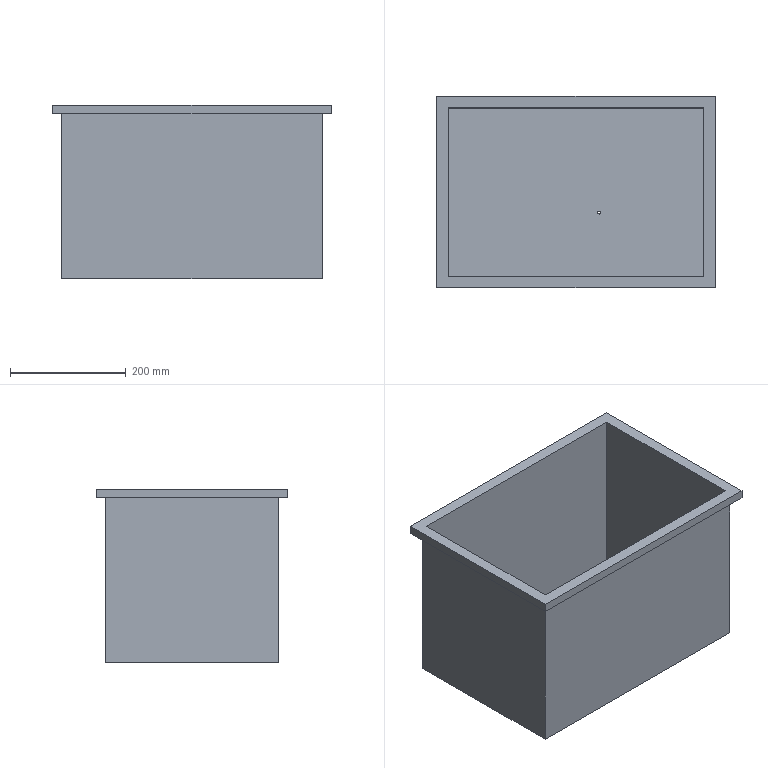Part | STEP file | Material box | 1 solid | 18 faces | box 480 x 330 x 300 mm | volume 3208902 mm3 | plane 16 | cylinder 2 | commonest cylinder face diameters 5 x2
STEP:
#1=CARTESIAN_POINT('',(0.,0.,0.));
#2=DIRECTION('',(0.,0.,1.));
#3=DIRECTION('',(1.,0.,0.));
#4=AXIS2_PLACEMENT_3D('',#1,#2,#3);
#5=CARTESIAN_POINT('',(42.5,-35.,0.));
#6=VERTEX_POINT('',#5);
#7=CARTESIAN_POINT('',(42.5,-35.,5.));
#8=VERTEX_POINT('',#7);
#9=CARTESIAN_POINT('',(42.5,-35.,-5.));
#10=DIRECTION('',(0.,0.,1.));
#11=VECTOR('',#10,1.);
#12=LINE('',#9,#11);
#13=CARTESIAN_POINT('',(40.,-35.,-5.));
#14=DIRECTION('',(0.,0.,1.));
#15=DIRECTION('',(1.,0.,0.));
#16=AXIS2_PLACEMENT_3D('',#13,#14,#15);
#17=CYLINDRICAL_SURFACE('',#16,2.5);
#18=CARTESIAN_POINT('',(6.283,0.));
#19=DIRECTION('',(0.,1.));
#20=VECTOR('',#19,1.);
#21=LINE('',#18,#20);
#22=(GEOMETRIC_REPRESENTATION_CONTEXT(2)PARAMETRIC_REPRESENTATION_CONTEXT()REPRESENTATION_CONTEXT('',''));
#23=DEFINITIONAL_REPRESENTATION('',(#21),#22);
#24=PCURVE('',#17,#23);
#25=CARTESIAN_POINT('',(40.,-35.,-5.));
#26=DIRECTION('',(0.,0.,1.));
#27=DIRECTION('',(1.,0.,0.));
#28=AXIS2_PLACEMENT_3D('',#25,#26,#27);
#29=CYLINDRICAL_SURFACE('',#28,2.5);
#30=CARTESIAN_POINT('',(0.,0.));
#31=DIRECTION('',(0.,1.));
#32=VECTOR('',#31,1.);
#33=LINE('',#30,#32);
#34=(GEOMETRIC_REPRESENTATION_CONTEXT(2)PARAMETRIC_REPRESENTATION_CONTEXT()REPRESENTATION_CONTEXT('',''));
#35=DEFINITIONAL_REPRESENTATION('',(#33),#34);
#36=PCURVE('',#29,#35);
#37=SURFACE_CURVE('',#12,(#24,#36),.PCURVE_S1.);
#38=EDGE_CURVE('',#6,#8,#37,.T.);
#39=ORIENTED_EDGE('',*,*,#38,.T.);
#40=CARTESIAN_POINT('',(37.5,-35.,5.));
#41=VERTEX_POINT('',#40);
#42=CARTESIAN_POINT('',(40.,-35.,5.));
#43=DIRECTION('',(0.,0.,-1.));
#44=DIRECTION('',(1.,0.,0.));
#45=AXIS2_PLACEMENT_3D('',#42,#43,#44);
#46=CIRCLE('',#45,2.5);
#47=CARTESIAN_POINT('',(6.283,10.));
#48=DIRECTION('',(-1.,0.));
#49=VECTOR('',#48,1.);
#50=LINE('',#47,#49);
#51=(GEOMETRIC_REPRESENTATION_CONTEXT(2)PARAMETRIC_REPRESENTATION_CONTEXT()REPRESENTATION_CONTEXT('',''));
#52=DEFINITIONAL_REPRESENTATION('',(#50),#51);
#53=PCURVE('',#17,#52);
#54=CARTESIAN_POINT('',(0.,0.,5.));
#55=DIRECTION('',(0.,0.,1.));
#56=DIRECTION('',(1.,0.,0.));
#57=AXIS2_PLACEMENT_3D('',#54,#55,#56);
#58=PLANE('',#57);
#59=CARTESIAN_POINT('',(42.5,-35.));
#60=CARTESIAN_POINT('',(42.5,-39.33));
#61=CARTESIAN_POINT('',(38.75,-37.165));
#62=CARTESIAN_POINT('',(35.,-35.));
#63=CARTESIAN_POINT('',(38.75,-32.835));
#64=CARTESIAN_POINT('',(42.5,-30.67));
#65=CARTESIAN_POINT('',(42.5,-35.));
#66=(BOUNDED_CURVE()B_SPLINE_CURVE(2,(#59,#60,#61,#62,#63,#64,#65),.UNSPECIFIED.,.T.,.F.)B_SPLINE_CURVE_WITH_KNOTS((1,2,2,2,2,1),(-2.094,0.,2.094,4.189,6.283,8.378),.UNSPECIFIED.)CURVE()GEOMETRIC_REPRESENTATION_ITEM()RATIONAL_B_SPLINE_CURVE((1.,0.5,1.,0.5,1.,0.5,1.))REPRESENTATION_ITEM(''));
#67=(GEOMETRIC_REPRESENTATION_CONTEXT(2)PARAMETRIC_REPRESENTATION_CONTEXT()REPRESENTATION_CONTEXT('',''));
#68=DEFINITIONAL_REPRESENTATION('',(#66),#67);
#69=PCURVE('',#58,#68);
#70=SURFACE_CURVE('',#46,(#53,#69),.PCURVE_S1.);
#71=EDGE_CURVE('',#8,#41,#70,.T.);
#72=ORIENTED_EDGE('',*,*,#71,.T.);
#73=CARTESIAN_POINT('',(37.5,-35.,0.));
#74=VERTEX_POINT('',#73);
#75=CARTESIAN_POINT('',(37.5,-35.,-5.));
#76=DIRECTION('',(0.,0.,1.));
#77=VECTOR('',#76,1.);
#78=LINE('',#75,#77);
#79=CARTESIAN_POINT('',(3.142,0.));
#80=DIRECTION('',(0.,1.));
#81=VECTOR('',#80,1.);
#82=LINE('',#79,#81);
#83=(GEOMETRIC_REPRESENTATION_CONTEXT(2)PARAMETRIC_REPRESENTATION_CONTEXT()REPRESENTATION_CONTEXT('',''));
#84=DEFINITIONAL_REPRESENTATION('',(#82),#83);
#85=PCURVE('',#17,#84);
#86=CARTESIAN_POINT('',(3.142,0.));
#87=DIRECTION('',(0.,1.));
#88=VECTOR('',#87,1.);
#89=LINE('',#86,#88);
#90=(GEOMETRIC_REPRESENTATION_CONTEXT(2)PARAMETRIC_REPRESENTATION_CONTEXT()REPRESENTATION_CONTEXT('',''));
#91=DEFINITIONAL_REPRESENTATION('',(#89),#90);
#92=PCURVE('',#29,#91);
#93=SURFACE_CURVE('',#78,(#85,#92),.PCURVE_S1.);
#94=EDGE_CURVE('',#74,#41,#93,.T.);
#95=ORIENTED_EDGE('',*,*,#94,.F.);
#96=CARTESIAN_POINT('',(40.,-35.,0.));
#97=DIRECTION('',(0.,0.,-1.));
#98=DIRECTION('',(1.,0.,0.));
#99=AXIS2_PLACEMENT_3D('',#96,#97,#98);
#100=CIRCLE('',#99,2.5);
#101=CARTESIAN_POINT('',(6.283,5.));
#102=DIRECTION('',(-1.,0.));
#103=VECTOR('',#102,1.);
#104=LINE('',#101,#103);
#105=(GEOMETRIC_REPRESENTATION_CONTEXT(2)PARAMETRIC_REPRESENTATION_CONTEXT()REPRESENTATION_CONTEXT('',''));
#106=DEFINITIONAL_REPRESENTATION('',(#104),#105);
#107=PCURVE('',#17,#106);
#108=CARTESIAN_POINT('',(0.,0.,0.));
#109=DIRECTION('',(0.,0.,1.));
#110=DIRECTION('',(1.,0.,0.));
#111=AXIS2_PLACEMENT_3D('',#108,#109,#110);
#112=PLANE('',#111);
#113=CARTESIAN_POINT('',(42.5,-35.));
#114=CARTESIAN_POINT('',(42.5,-39.33));
#115=CARTESIAN_POINT('',(38.75,-37.165));
#116=CARTESIAN_POINT('',(35.,-35.));
#117=CARTESIAN_POINT('',(38.75,-32.835));
#118=CARTESIAN_POINT('',(42.5,-30.67));
#119=CARTESIAN_POINT('',(42.5,-35.));
#120=(BOUNDED_CURVE()B_SPLINE_CURVE(2,(#113,#114,#115,#116,#117,#118,#119),.UNSPECIFIED.,.T.,.F.)B_SPLINE_CURVE_WITH_KNOTS((1,2,2,2,2,1),(-2.094,0.,2.094,4.189,6.283,8.378),.UNSPECIFIED.)CURVE()GEOMETRIC_REPRESENTATION_ITEM()RATIONAL_B_SPLINE_CURVE((1.,0.5,1.,0.5,1.,0.5,1.))REPRESENTATION_ITEM(''));
#121=(GEOMETRIC_REPRESENTATION_CONTEXT(2)PARAMETRIC_REPRESENTATION_CONTEXT()REPRESENTATION_CONTEXT('',''));
#122=DEFINITIONAL_REPRESENTATION('',(#120),#121);
#123=PCURVE('',#112,#122);
#124=SURFACE_CURVE('',#100,(#107,#123),.PCURVE_S1.);
#125=EDGE_CURVE('',#6,#74,#124,.T.);
#126=ORIENTED_EDGE('',*,*,#125,.F.);
#127=EDGE_LOOP('',(#39,#72,#95,#126));
#128=FACE_BOUND('',#127,.F.);
#129=ADVANCED_FACE('',(#128),#17,.F.);
#130=CARTESIAN_POINT('',(-225.,-150.,0.));
#131=VERTEX_POINT('',#130);
#132=CARTESIAN_POINT('',(225.,-150.,0.));
#133=VERTEX_POINT('',#132);
#134=CARTESIAN_POINT('',(0.,-150.,0.));
#135=DIRECTION('',(1.,0.,0.));
#136=VECTOR('',#135,1.);
#137=LINE('',#134,#136);
#138=CARTESIAN_POINT('',(0.,-150.));
#139=DIRECTION('',(1.,0.));
#140=VECTOR('',#139,1.);
#141=LINE('',#138,#140);
#142=(GEOMETRIC_REPRESENTATION_CONTEXT(2)PARAMETRIC_REPRESENTATION_CONTEXT()REPRESENTATION_CONTEXT('',''));
#143=DEFINITIONAL_REPRESENTATION('',(#141),#142);
#144=PCURVE('',#112,#143);
#145=CARTESIAN_POINT('',(-225.,-150.,300.));
#146=DIRECTION('',(0.,1.,0.));
#147=DIRECTION('',(0.,0.,1.));
#148=AXIS2_PLACEMENT_3D('',#145,#146,#147);
#149=PLANE('',#148);
#150=CARTESIAN_POINT('',(-300.,225.));
#151=DIRECTION('',(0.,1.));
#152=VECTOR('',#151,1.);
#153=LINE('',#150,#152);
#154=(GEOMETRIC_REPRESENTATION_CONTEXT(2)PARAMETRIC_REPRESENTATION_CONTEXT()REPRESENTATION_CONTEXT('',''));
#155=DEFINITIONAL_REPRESENTATION('',(#153),#154);
#156=PCURVE('',#149,#155);
#157=SURFACE_CURVE('',#137,(#144,#156),.PCURVE_S1.);
#158=EDGE_CURVE('',#131,#133,#157,.T.);
#159=ORIENTED_EDGE('',*,*,#158,.F.);
#160=CARTESIAN_POINT('',(-225.,150.,0.));
#161=VERTEX_POINT('',#160);
#162=CARTESIAN_POINT('',(-225.,0.,0.));
#163=DIRECTION('',(0.,-1.,0.));
#164=VECTOR('',#163,1.);
#165=LINE('',#162,#164);
#166=CARTESIAN_POINT('',(-225.,0.));
#167=DIRECTION('',(0.,-1.));
#168=VECTOR('',#167,1.);
#169=LINE('',#166,#168);
#170=(GEOMETRIC_REPRESENTATION_CONTEXT(2)PARAMETRIC_REPRESENTATION_CONTEXT()REPRESENTATION_CONTEXT('',''));
#171=DEFINITIONAL_REPRESENTATION('',(#169),#170);
#172=PCURVE('',#112,#171);
#173=CARTESIAN_POINT('',(-225.,150.,300.));
#174=DIRECTION('',(1.,0.,0.));
#175=DIRECTION('',(0.,1.,0.));
#176=AXIS2_PLACEMENT_3D('',#173,#174,#175);
#177=PLANE('',#176);
#178=CARTESIAN_POINT('',(-150.,-300.));
#179=DIRECTION('',(-1.,0.));
#180=VECTOR('',#179,1.);
#181=LINE('',#178,#180);
#182=(GEOMETRIC_REPRESENTATION_CONTEXT(2)PARAMETRIC_REPRESENTATION_CONTEXT()REPRESENTATION_CONTEXT('',''));
#183=DEFINITIONAL_REPRESENTATION('',(#181),#182);
#184=PCURVE('',#177,#183);
#185=SURFACE_CURVE('',#165,(#172,#184),.PCURVE_S1.);
#186=EDGE_CURVE('',#161,#131,#185,.T.);
#187=ORIENTED_EDGE('',*,*,#186,.F.);
#188=CARTESIAN_POINT('',(225.,150.,0.));
#189=VERTEX_POINT('',#188);
#190=CARTESIAN_POINT('',(0.,150.,0.));
#191=DIRECTION('',(-1.,0.,0.));
#192=VECTOR('',#191,1.);
#193=LINE('',#190,#192);
#194=CARTESIAN_POINT('',(0.,150.));
#195=DIRECTION('',(-1.,0.));
#196=VECTOR('',#195,1.);
#197=LINE('',#194,#196);
#198=(GEOMETRIC_REPRESENTATION_CONTEXT(2)PARAMETRIC_REPRESENTATION_CONTEXT()REPRESENTATION_CONTEXT('',''));
#199=DEFINITIONAL_REPRESENTATION('',(#197),#198);
#200=PCURVE('',#112,#199);
#201=CARTESIAN_POINT('',(-225.,150.,300.));
#202=DIRECTION('',(0.,-1.,0.));
#203=DIRECTION('',(0.,0.,-1.));
#204=AXIS2_PLACEMENT_3D('',#201,#202,#203);
#205=PLANE('',#204);
#206=CARTESIAN_POINT('',(300.,225.));
#207=DIRECTION('',(0.,-1.));
#208=VECTOR('',#207,1.);
#209=LINE('',#206,#208);
#210=(GEOMETRIC_REPRESENTATION_CONTEXT(2)PARAMETRIC_REPRESENTATION_CONTEXT()REPRESENTATION_CONTEXT('',''));
#211=DEFINITIONAL_REPRESENTATION('',(#209),#210);
#212=PCURVE('',#205,#211);
#213=SURFACE_CURVE('',#193,(#200,#212),.PCURVE_S1.);
#214=EDGE_CURVE('',#189,#161,#213,.T.);
#215=ORIENTED_EDGE('',*,*,#214,.F.);
#216=CARTESIAN_POINT('',(225.,0.,0.));
#217=DIRECTION('',(0.,1.,0.));
#218=VECTOR('',#217,1.);
#219=LINE('',#216,#218);
#220=CARTESIAN_POINT('',(225.,0.));
#221=DIRECTION('',(0.,1.));
#222=VECTOR('',#221,1.);
#223=LINE('',#220,#222);
#224=(GEOMETRIC_REPRESENTATION_CONTEXT(2)PARAMETRIC_REPRESENTATION_CONTEXT()REPRESENTATION_CONTEXT('',''));
#225=DEFINITIONAL_REPRESENTATION('',(#223),#224);
#226=PCURVE('',#112,#225);
#227=CARTESIAN_POINT('',(225.,150.,300.));
#228=DIRECTION('',(-1.,0.,0.));
#229=DIRECTION('',(0.,-1.,0.));
#230=AXIS2_PLACEMENT_3D('',#227,#228,#229);
#231=PLANE('',#230);
#232=CARTESIAN_POINT('',(150.,-300.));
#233=DIRECTION('',(-1.,0.));
#234=VECTOR('',#233,1.);
#235=LINE('',#232,#234);
#236=(GEOMETRIC_REPRESENTATION_CONTEXT(2)PARAMETRIC_REPRESENTATION_CONTEXT()REPRESENTATION_CONTEXT('',''));
#237=DEFINITIONAL_REPRESENTATION('',(#235),#236);
#238=PCURVE('',#231,#237);
#239=SURFACE_CURVE('',#219,(#226,#238),.PCURVE_S1.);
#240=EDGE_CURVE('',#133,#189,#239,.T.);
#241=ORIENTED_EDGE('',*,*,#240,.F.);
#242=EDGE_LOOP('',(#159,#187,#215,#241));
#243=FACE_BOUND('',#242,.T.);
#244=ORIENTED_EDGE('',*,*,#125,.F.);
#245=CARTESIAN_POINT('',(40.,-35.,0.));
#246=DIRECTION('',(0.,0.,-1.));
#247=DIRECTION('',(1.,0.,0.));
#248=AXIS2_PLACEMENT_3D('',#245,#246,#247);
#249=CIRCLE('',#248,2.5);
#250=CARTESIAN_POINT('',(42.5,-35.));
#251=CARTESIAN_POINT('',(42.5,-39.33));
#252=CARTESIAN_POINT('',(38.75,-37.165));
#253=CARTESIAN_POINT('',(35.,-35.));
#254=CARTESIAN_POINT('',(38.75,-32.835));
#255=CARTESIAN_POINT('',(42.5,-30.67));
#256=CARTESIAN_POINT('',(42.5,-35.));
#257=(BOUNDED_CURVE()B_SPLINE_CURVE(2,(#250,#251,#252,#253,#254,#255,#256),.UNSPECIFIED.,.T.,.F.)B_SPLINE_CURVE_WITH_KNOTS((1,2,2,2,2,1),(-2.094,0.,2.094,4.189,6.283,8.378),.UNSPECIFIED.)CURVE()GEOMETRIC_REPRESENTATION_ITEM()RATIONAL_B_SPLINE_CURVE((1.,0.5,1.,0.5,1.,0.5,1.))REPRESENTATION_ITEM(''));
#258=(GEOMETRIC_REPRESENTATION_CONTEXT(2)PARAMETRIC_REPRESENTATION_CONTEXT()REPRESENTATION_CONTEXT('',''));
#259=DEFINITIONAL_REPRESENTATION('',(#257),#258);
#260=PCURVE('',#112,#259);
#261=CARTESIAN_POINT('',(6.283,5.));
#262=DIRECTION('',(-1.,0.));
#263=VECTOR('',#262,1.);
#264=LINE('',#261,#263);
#265=(GEOMETRIC_REPRESENTATION_CONTEXT(2)PARAMETRIC_REPRESENTATION_CONTEXT()REPRESENTATION_CONTEXT('',''));
#266=DEFINITIONAL_REPRESENTATION('',(#264),#265);
#267=PCURVE('',#29,#266);
#268=SURFACE_CURVE('',#249,(#260,#267),.PCURVE_S1.);
#269=EDGE_CURVE('',#74,#6,#268,.T.);
#270=ORIENTED_EDGE('',*,*,#269,.F.);
#271=EDGE_LOOP('',(#244,#270));
#272=FACE_BOUND('',#271,.T.);
#273=ADVANCED_FACE('',(#243,#272),#112,.F.);
#274=CARTESIAN_POINT('',(225.,-150.,285.));
#275=VERTEX_POINT('',#274);
#276=CARTESIAN_POINT('',(225.,150.,285.));
#277=VERTEX_POINT('',#276);
#278=CARTESIAN_POINT('',(225.,150.,285.));
#279=DIRECTION('',(0.,1.,0.));
#280=VECTOR('',#279,1.);
#281=LINE('',#278,#280);
#282=CARTESIAN_POINT('',(0.,-15.));
#283=DIRECTION('',(-1.,0.));
#284=VECTOR('',#283,1.);
#285=LINE('',#282,#284);
#286=(GEOMETRIC_REPRESENTATION_CONTEXT(2)PARAMETRIC_REPRESENTATION_CONTEXT()REPRESENTATION_CONTEXT('',''));
#287=DEFINITIONAL_REPRESENTATION('',(#285),#286);
#288=PCURVE('',#231,#287);
#289=CARTESIAN_POINT('',(0.,0.,285.));
#290=DIRECTION('',(0.,0.,-1.));
#291=DIRECTION('',(-1.,0.,0.));
#292=AXIS2_PLACEMENT_3D('',#289,#290,#291);
#293=PLANE('',#292);
#294=CARTESIAN_POINT('',(-225.,150.));
#295=DIRECTION('',(0.,1.));
#296=VECTOR('',#295,1.);
#297=LINE('',#294,#296);
#298=(GEOMETRIC_REPRESENTATION_CONTEXT(2)PARAMETRIC_REPRESENTATION_CONTEXT()REPRESENTATION_CONTEXT('',''));
#299=DEFINITIONAL_REPRESENTATION('',(#297),#298);
#300=PCURVE('',#293,#299);
#301=SURFACE_CURVE('',#281,(#288,#300),.PCURVE_S1.);
#302=EDGE_CURVE('',#275,#277,#301,.T.);
#303=ORIENTED_EDGE('',*,*,#302,.F.);
#304=CARTESIAN_POINT('',(225.,-150.,300.));
#305=DIRECTION('',(0.,0.,1.));
#306=VECTOR('',#305,1.);
#307=LINE('',#304,#306);
#308=CARTESIAN_POINT('',(300.,0.));
#309=DIRECTION('',(0.,1.));
#310=VECTOR('',#309,1.);
#311=LINE('',#308,#310);
#312=(GEOMETRIC_REPRESENTATION_CONTEXT(2)PARAMETRIC_REPRESENTATION_CONTEXT()REPRESENTATION_CONTEXT('',''));
#313=DEFINITIONAL_REPRESENTATION('',(#311),#312);
#314=PCURVE('',#231,#313);
#315=CARTESIAN_POINT('',(0.,450.));
#316=DIRECTION('',(1.,0.));
#317=VECTOR('',#316,1.);
#318=LINE('',#315,#317);
#319=(GEOMETRIC_REPRESENTATION_CONTEXT(2)PARAMETRIC_REPRESENTATION_CONTEXT()REPRESENTATION_CONTEXT('',''));
#320=DEFINITIONAL_REPRESENTATION('',(#318),#319);
#321=PCURVE('',#149,#320);
#322=SURFACE_CURVE('',#307,(#314,#321),.PCURVE_S1.);
#323=EDGE_CURVE('',#133,#275,#322,.T.);
#324=ORIENTED_EDGE('',*,*,#323,.F.);
#325=ORIENTED_EDGE('',*,*,#240,.T.);
#326=CARTESIAN_POINT('',(225.,150.,300.));
#327=DIRECTION('',(0.,0.,-1.));
#328=VECTOR('',#327,1.);
#329=LINE('',#326,#328);
#330=CARTESIAN_POINT('',(0.,0.));
#331=DIRECTION('',(0.,-1.));
#332=VECTOR('',#331,1.);
#333=LINE('',#330,#332);
#334=(GEOMETRIC_REPRESENTATION_CONTEXT(2)PARAMETRIC_REPRESENTATION_CONTEXT()REPRESENTATION_CONTEXT('',''));
#335=DEFINITIONAL_REPRESENTATION('',(#333),#334);
#336=PCURVE('',#231,#335);
#337=CARTESIAN_POINT('',(0.,450.));
#338=DIRECTION('',(1.,0.));
#339=VECTOR('',#338,1.);
#340=LINE('',#337,#339);
#341=(GEOMETRIC_REPRESENTATION_CONTEXT(2)PARAMETRIC_REPRESENTATION_CONTEXT()REPRESENTATION_CONTEXT('',''));
#342=DEFINITIONAL_REPRESENTATION('',(#340),#341);
#343=PCURVE('',#205,#342);
#344=SURFACE_CURVE('',#329,(#336,#343),.PCURVE_S1.);
#345=EDGE_CURVE('',#277,#189,#344,.T.);
#346=ORIENTED_EDGE('',*,*,#345,.F.);
#347=EDGE_LOOP('',(#303,#324,#325,#346));
#348=FACE_BOUND('',#347,.T.);
#349=ADVANCED_FACE('',(#348),#231,.F.);
#350=CARTESIAN_POINT('',(-225.,-150.,285.));
#351=VERTEX_POINT('',#350);
#352=CARTESIAN_POINT('',(-225.,-150.,285.));
#353=DIRECTION('',(1.,0.,0.));
#354=VECTOR('',#353,1.);
#355=LINE('',#352,#354);
#356=CARTESIAN_POINT('',(-15.,0.));
#357=DIRECTION('',(0.,1.));
#358=VECTOR('',#357,1.);
#359=LINE('',#356,#358);
#360=(GEOMETRIC_REPRESENTATION_CONTEXT(2)PARAMETRIC_REPRESENTATION_CONTEXT()REPRESENTATION_CONTEXT('',''));
#361=DEFINITIONAL_REPRESENTATION('',(#359),#360);
#362=PCURVE('',#149,#361);
#363=CARTESIAN_POINT('',(225.,-150.));
#364=DIRECTION('',(-1.,0.));
#365=VECTOR('',#364,1.);
#366=LINE('',#363,#365);
#367=(GEOMETRIC_REPRESENTATION_CONTEXT(2)PARAMETRIC_REPRESENTATION_CONTEXT()REPRESENTATION_CONTEXT('',''));
#368=DEFINITIONAL_REPRESENTATION('',(#366),#367);
#369=PCURVE('',#293,#368);
#370=SURFACE_CURVE('',#355,(#362,#369),.PCURVE_S1.);
#371=EDGE_CURVE('',#351,#275,#370,.T.);
#372=ORIENTED_EDGE('',*,*,#371,.F.);
#373=CARTESIAN_POINT('',(-225.,-150.,300.));
#374=DIRECTION('',(0.,0.,1.));
#375=VECTOR('',#374,1.);
#376=LINE('',#373,#375);
#377=CARTESIAN_POINT('',(0.,0.));
#378=DIRECTION('',(1.,0.));
#379=VECTOR('',#378,1.);
#380=LINE('',#377,#379);
#381=(GEOMETRIC_REPRESENTATION_CONTEXT(2)PARAMETRIC_REPRESENTATION_CONTEXT()REPRESENTATION_CONTEXT('',''));
#382=DEFINITIONAL_REPRESENTATION('',(#380),#381);
#383=PCURVE('',#149,#382);
#384=CARTESIAN_POINT('',(-300.,0.));
#385=DIRECTION('',(0.,1.));
#386=VECTOR('',#385,1.);
#387=LINE('',#384,#386);
#388=(GEOMETRIC_REPRESENTATION_CONTEXT(2)PARAMETRIC_REPRESENTATION_CONTEXT()REPRESENTATION_CONTEXT('',''));
#389=DEFINITIONAL_REPRESENTATION('',(#387),#388);
#390=PCURVE('',#177,#389);
#391=SURFACE_CURVE('',#376,(#383,#390),.PCURVE_S1.);
#392=EDGE_CURVE('',#131,#351,#391,.T.);
#393=ORIENTED_EDGE('',*,*,#392,.F.);
#394=ORIENTED_EDGE('',*,*,#158,.T.);
#395=ORIENTED_EDGE('',*,*,#323,.T.);
#396=EDGE_LOOP('',(#372,#393,#394,#395));
#397=FACE_BOUND('',#396,.T.);
#398=ADVANCED_FACE('',(#397),#149,.F.);
#399=CARTESIAN_POINT('',(-225.,150.,285.));
#400=VERTEX_POINT('',#399);
#401=CARTESIAN_POINT('',(-225.,150.,285.));
#402=DIRECTION('',(0.,-1.,0.));
#403=VECTOR('',#402,1.);
#404=LINE('',#401,#403);
#405=CARTESIAN_POINT('',(0.,-15.));
#406=DIRECTION('',(-1.,0.));
#407=VECTOR('',#406,1.);
#408=LINE('',#405,#407);
#409=(GEOMETRIC_REPRESENTATION_CONTEXT(2)PARAMETRIC_REPRESENTATION_CONTEXT()REPRESENTATION_CONTEXT('',''));
#410=DEFINITIONAL_REPRESENTATION('',(#408),#409);
#411=PCURVE('',#177,#410);
#412=CARTESIAN_POINT('',(225.,150.));
#413=DIRECTION('',(0.,-1.));
#414=VECTOR('',#413,1.);
#415=LINE('',#412,#414);
#416=(GEOMETRIC_REPRESENTATION_CONTEXT(2)PARAMETRIC_REPRESENTATION_CONTEXT()REPRESENTATION_CONTEXT('',''));
#417=DEFINITIONAL_REPRESENTATION('',(#415),#416);
#418=PCURVE('',#293,#417);
#419=SURFACE_CURVE('',#404,(#411,#418),.PCURVE_S1.);
#420=EDGE_CURVE('',#400,#351,#419,.T.);
#421=ORIENTED_EDGE('',*,*,#420,.F.);
#422=CARTESIAN_POINT('',(-225.,150.,300.));
#423=DIRECTION('',(0.,0.,1.));
#424=VECTOR('',#423,1.);
#425=LINE('',#422,#424);
#426=CARTESIAN_POINT('',(0.,0.));
#427=DIRECTION('',(0.,1.));
#428=VECTOR('',#427,1.);
#429=LINE('',#426,#428);
#430=(GEOMETRIC_REPRESENTATION_CONTEXT(2)PARAMETRIC_REPRESENTATION_CONTEXT()REPRESENTATION_CONTEXT('',''));
#431=DEFINITIONAL_REPRESENTATION('',(#429),#430);
#432=PCURVE('',#177,#431);
#433=CARTESIAN_POINT('',(0.,0.));
#434=DIRECTION('',(-1.,0.));
#435=VECTOR('',#434,1.);
#436=LINE('',#433,#435);
#437=(GEOMETRIC_REPRESENTATION_CONTEXT(2)PARAMETRIC_REPRESENTATION_CONTEXT()REPRESENTATION_CONTEXT('',''));
#438=DEFINITIONAL_REPRESENTATION('',(#436),#437);
#439=PCURVE('',#205,#438);
#440=SURFACE_CURVE('',#425,(#432,#439),.PCURVE_S1.);
#441=EDGE_CURVE('',#161,#400,#440,.T.);
#442=ORIENTED_EDGE('',*,*,#441,.F.);
#443=ORIENTED_EDGE('',*,*,#186,.T.);
#444=ORIENTED_EDGE('',*,*,#392,.T.);
#445=EDGE_LOOP('',(#421,#442,#443,#444));
#446=FACE_BOUND('',#445,.T.);
#447=ADVANCED_FACE('',(#446),#177,.F.);
#448=CARTESIAN_POINT('',(-225.,150.,285.));
#449=DIRECTION('',(-1.,0.,0.));
#450=VECTOR('',#449,1.);
#451=LINE('',#448,#450);
#452=CARTESIAN_POINT('',(15.,0.));
#453=DIRECTION('',(0.,-1.));
#454=VECTOR('',#453,1.);
#455=LINE('',#452,#454);
#456=(GEOMETRIC_REPRESENTATION_CONTEXT(2)PARAMETRIC_REPRESENTATION_CONTEXT()REPRESENTATION_CONTEXT('',''));
#457=DEFINITIONAL_REPRESENTATION('',(#455),#456);
#458=PCURVE('',#205,#457);
#459=CARTESIAN_POINT('',(225.,150.));
#460=DIRECTION('',(1.,0.));
#461=VECTOR('',#460,1.);
#462=LINE('',#459,#461);
#463=(GEOMETRIC_REPRESENTATION_CONTEXT(2)PARAMETRIC_REPRESENTATION_CONTEXT()REPRESENTATION_CONTEXT('',''));
#464=DEFINITIONAL_REPRESENTATION('',(#462),#463);
#465=PCURVE('',#293,#464);
#466=SURFACE_CURVE('',#451,(#458,#465),.PCURVE_S1.);
#467=EDGE_CURVE('',#277,#400,#466,.T.);
#468=ORIENTED_EDGE('',*,*,#467,.F.);
#469=ORIENTED_EDGE('',*,*,#345,.T.);
#470=ORIENTED_EDGE('',*,*,#214,.T.);
#471=ORIENTED_EDGE('',*,*,#441,.T.);
#472=EDGE_LOOP('',(#468,#469,#470,#471));
#473=FACE_BOUND('',#472,.T.);
#474=ADVANCED_FACE('',(#473),#205,.F.);
#475=CARTESIAN_POINT('',(40.,-35.,5.));
#476=DIRECTION('',(0.,0.,-1.));
#477=DIRECTION('',(1.,0.,0.));
#478=AXIS2_PLACEMENT_3D('',#475,#476,#477);
#479=CIRCLE('',#478,2.5);
#480=CARTESIAN_POINT('',(6.283,10.));
#481=DIRECTION('',(-1.,0.));
#482=VECTOR('',#481,1.);
#483=LINE('',#480,#482);
#484=(GEOMETRIC_REPRESENTATION_CONTEXT(2)PARAMETRIC_REPRESENTATION_CONTEXT()REPRESENTATION_CONTEXT('',''));
#485=DEFINITIONAL_REPRESENTATION('',(#483),#484);
#486=PCURVE('',#29,#485);
#487=CARTESIAN_POINT('',(42.5,-35.));
#488=CARTESIAN_POINT('',(42.5,-39.33));
#489=CARTESIAN_POINT('',(38.75,-37.165));
#490=CARTESIAN_POINT('',(35.,-35.));
#491=CARTESIAN_POINT('',(38.75,-32.835));
#492=CARTESIAN_POINT('',(42.5,-30.67));
#493=CARTESIAN_POINT('',(42.5,-35.));
#494=(BOUNDED_CURVE()B_SPLINE_CURVE(2,(#487,#488,#489,#490,#491,#492,#493),.UNSPECIFIED.,.T.,.F.)B_SPLINE_CURVE_WITH_KNOTS((1,2,2,2,2,1),(-2.094,0.,2.094,4.189,6.283,8.378),.UNSPECIFIED.)CURVE()GEOMETRIC_REPRESENTATION_ITEM()RATIONAL_B_SPLINE_CURVE((1.,0.5,1.,0.5,1.,0.5,1.))REPRESENTATION_ITEM(''));
#495=(GEOMETRIC_REPRESENTATION_CONTEXT(2)PARAMETRIC_REPRESENTATION_CONTEXT()REPRESENTATION_CONTEXT('',''));
#496=DEFINITIONAL_REPRESENTATION('',(#494),#495);
#497=PCURVE('',#58,#496);
#498=SURFACE_CURVE('',#479,(#486,#497),.PCURVE_S1.);
#499=EDGE_CURVE('',#41,#8,#498,.T.);
#500=ORIENTED_EDGE('',*,*,#499,.T.);
#501=ORIENTED_EDGE('',*,*,#38,.F.);
#502=ORIENTED_EDGE('',*,*,#269,.F.);
#503=ORIENTED_EDGE('',*,*,#94,.T.);
#504=EDGE_LOOP('',(#500,#501,#502,#503));
#505=FACE_BOUND('',#504,.F.);
#506=ADVANCED_FACE('',(#505),#29,.F.);
#507=CARTESIAN_POINT('',(240.,-165.,285.));
#508=VERTEX_POINT('',#507);
#509=CARTESIAN_POINT('',(-240.,-165.,285.));
#510=VERTEX_POINT('',#509);
#511=CARTESIAN_POINT('',(0.,-165.,285.));
#512=DIRECTION('',(-1.,0.,0.));
#513=VECTOR('',#512,1.);
#514=LINE('',#511,#513);
#515=CARTESIAN_POINT('',(0.,-165.));
#516=DIRECTION('',(1.,0.));
#517=VECTOR('',#516,1.);
#518=LINE('',#515,#517);
#519=(GEOMETRIC_REPRESENTATION_CONTEXT(2)PARAMETRIC_REPRESENTATION_CONTEXT()REPRESENTATION_CONTEXT('',''));
#520=DEFINITIONAL_REPRESENTATION('',(#518),#519);
#521=PCURVE('',#293,#520);
#522=CARTESIAN_POINT('',(-240.,-165.,285.));
#523=DIRECTION('',(0.,-1.,0.));
#524=DIRECTION('',(0.,0.,-1.));
#525=AXIS2_PLACEMENT_3D('',#522,#523,#524);
#526=PLANE('',#525);
#527=CARTESIAN_POINT('',(0.,240.));
#528=DIRECTION('',(0.,-1.));
#529=VECTOR('',#528,1.);
#530=LINE('',#527,#529);
#531=(GEOMETRIC_REPRESENTATION_CONTEXT(2)PARAMETRIC_REPRESENTATION_CONTEXT()REPRESENTATION_CONTEXT('',''));
#532=DEFINITIONAL_REPRESENTATION('',(#530),#531);
#533=PCURVE('',#526,#532);
#534=SURFACE_CURVE('',#514,(#521,#533),.PCURVE_S1.);
#535=EDGE_CURVE('',#508,#510,#534,.T.);
#536=ORIENTED_EDGE('',*,*,#535,.T.);
#537=CARTESIAN_POINT('',(-240.,165.,285.));
#538=VERTEX_POINT('',#537);
#539=CARTESIAN_POINT('',(-240.,0.,285.));
#540=DIRECTION('',(0.,1.,0.));
#541=VECTOR('',#540,1.);
#542=LINE('',#539,#541);
#543=CARTESIAN_POINT('',(240.,0.));
#544=DIRECTION('',(0.,1.));
#545=VECTOR('',#544,1.);
#546=LINE('',#543,#545);
#547=(GEOMETRIC_REPRESENTATION_CONTEXT(2)PARAMETRIC_REPRESENTATION_CONTEXT()REPRESENTATION_CONTEXT('',''));
#548=DEFINITIONAL_REPRESENTATION('',(#546),#547);
#549=PCURVE('',#293,#548);
#550=CARTESIAN_POINT('',(-240.,165.,285.));
#551=DIRECTION('',(-1.,0.,0.));
#552=DIRECTION('',(0.,-1.,0.));
#553=AXIS2_PLACEMENT_3D('',#550,#551,#552);
#554=PLANE('',#553);
#555=CARTESIAN_POINT('',(165.,0.));
#556=DIRECTION('',(-1.,0.));
#557=VECTOR('',#556,1.);
#558=LINE('',#555,#557);
#559=(GEOMETRIC_REPRESENTATION_CONTEXT(2)PARAMETRIC_REPRESENTATION_CONTEXT()REPRESENTATION_CONTEXT('',''));
#560=DEFINITIONAL_REPRESENTATION('',(#558),#559);
#561=PCURVE('',#554,#560);
#562=SURFACE_CURVE('',#542,(#549,#561),.PCURVE_S1.);
#563=EDGE_CURVE('',#510,#538,#562,.T.);
#564=ORIENTED_EDGE('',*,*,#563,.T.);
#565=CARTESIAN_POINT('',(240.,165.,285.));
#566=VERTEX_POINT('',#565);
#567=CARTESIAN_POINT('',(0.,165.,285.));
#568=DIRECTION('',(1.,0.,0.));
#569=VECTOR('',#568,1.);
#570=LINE('',#567,#569);
#571=CARTESIAN_POINT('',(0.,165.));
#572=DIRECTION('',(-1.,0.));
#573=VECTOR('',#572,1.);
#574=LINE('',#571,#573);
#575=(GEOMETRIC_REPRESENTATION_CONTEXT(2)PARAMETRIC_REPRESENTATION_CONTEXT()REPRESENTATION_CONTEXT('',''));
#576=DEFINITIONAL_REPRESENTATION('',(#574),#575);
#577=PCURVE('',#293,#576);
#578=CARTESIAN_POINT('',(-240.,165.,285.));
#579=DIRECTION('',(0.,1.,0.));
#580=DIRECTION('',(0.,0.,1.));
#581=AXIS2_PLACEMENT_3D('',#578,#579,#580);
#582=PLANE('',#581);
#583=CARTESIAN_POINT('',(0.,240.));
#584=DIRECTION('',(0.,1.));
#585=VECTOR('',#584,1.);
#586=LINE('',#583,#585);
#587=(GEOMETRIC_REPRESENTATION_CONTEXT(2)PARAMETRIC_REPRESENTATION_CONTEXT()REPRESENTATION_CONTEXT('',''));
#588=DEFINITIONAL_REPRESENTATION('',(#586),#587);
#589=PCURVE('',#582,#588);
#590=SURFACE_CURVE('',#570,(#577,#589),.PCURVE_S1.);
#591=EDGE_CURVE('',#538,#566,#590,.T.);
#592=ORIENTED_EDGE('',*,*,#591,.T.);
#593=CARTESIAN_POINT('',(240.,0.,285.));
#594=DIRECTION('',(0.,-1.,0.));
#595=VECTOR('',#594,1.);
#596=LINE('',#593,#595);
#597=CARTESIAN_POINT('',(-240.,0.));
#598=DIRECTION('',(0.,-1.));
#599=VECTOR('',#598,1.);
#600=LINE('',#597,#599);
#601=(GEOMETRIC_REPRESENTATION_CONTEXT(2)PARAMETRIC_REPRESENTATION_CONTEXT()REPRESENTATION_CONTEXT('',''));
#602=DEFINITIONAL_REPRESENTATION('',(#600),#601);
#603=PCURVE('',#293,#602);
#604=CARTESIAN_POINT('',(240.,165.,285.));
#605=DIRECTION('',(1.,0.,0.));
#606=DIRECTION('',(0.,0.,-1.));
#607=AXIS2_PLACEMENT_3D('',#604,#605,#606);
#608=PLANE('',#607);
#609=CARTESIAN_POINT('',(0.,-165.));
#610=DIRECTION('',(0.,-1.));
#611=VECTOR('',#610,1.);
#612=LINE('',#609,#611);
#613=(GEOMETRIC_REPRESENTATION_CONTEXT(2)PARAMETRIC_REPRESENTATION_CONTEXT()REPRESENTATION_CONTEXT('',''));
#614=DEFINITIONAL_REPRESENTATION('',(#612),#613);
#615=PCURVE('',#608,#614);
#616=SURFACE_CURVE('',#596,(#603,#615),.PCURVE_S1.);
#617=EDGE_CURVE('',#566,#508,#616,.T.);
#618=ORIENTED_EDGE('',*,*,#617,.T.);
#619=EDGE_LOOP('',(#536,#564,#592,#618));
#620=FACE_BOUND('',#619,.T.);
#621=ORIENTED_EDGE('',*,*,#302,.T.);
#622=ORIENTED_EDGE('',*,*,#467,.T.);
#623=ORIENTED_EDGE('',*,*,#420,.T.);
#624=ORIENTED_EDGE('',*,*,#371,.T.);
#625=EDGE_LOOP('',(#621,#622,#623,#624));
#626=FACE_BOUND('',#625,.T.);
#627=ADVANCED_FACE('',(#620,#626),#293,.T.);
#628=CARTESIAN_POINT('',(-220.,145.,5.));
#629=VERTEX_POINT('',#628);
#630=CARTESIAN_POINT('',(-220.,-145.,5.));
#631=VERTEX_POINT('',#630);
#632=CARTESIAN_POINT('',(-220.,0.,5.));
#633=DIRECTION('',(0.,-1.,0.));
#634=VECTOR('',#633,1.);
#635=LINE('',#632,#634);
#636=CARTESIAN_POINT('',(-220.,0.));
#637=DIRECTION('',(0.,-1.));
#638=VECTOR('',#637,1.);
#639=LINE('',#636,#638);
#640=(GEOMETRIC_REPRESENTATION_CONTEXT(2)PARAMETRIC_REPRESENTATION_CONTEXT()REPRESENTATION_CONTEXT('',''));
#641=DEFINITIONAL_REPRESENTATION('',(#639),#640);
#642=PCURVE('',#58,#641);
#643=CARTESIAN_POINT('',(-220.,150.,300.));
#644=DIRECTION('',(1.,0.,0.));
#645=DIRECTION('',(0.,1.,0.));
#646=AXIS2_PLACEMENT_3D('',#643,#644,#645);
#647=PLANE('',#646);
#648=CARTESIAN_POINT('',(-150.,-295.));
#649=DIRECTION('',(-1.,0.));
#650=VECTOR('',#649,1.);
#651=LINE('',#648,#650);
#652=(GEOMETRIC_REPRESENTATION_CONTEXT(2)PARAMETRIC_REPRESENTATION_CONTEXT()REPRESENTATION_CONTEXT('',''));
#653=DEFINITIONAL_REPRESENTATION('',(#651),#652);
#654=PCURVE('',#647,#653);
#655=SURFACE_CURVE('',#635,(#642,#654),.PCURVE_S1.);
#656=EDGE_CURVE('',#629,#631,#655,.T.);
#657=ORIENTED_EDGE('',*,*,#656,.T.);
#658=CARTESIAN_POINT('',(220.,-145.,5.));
#659=VERTEX_POINT('',#658);
#660=CARTESIAN_POINT('',(0.,-145.,5.));
#661=DIRECTION('',(1.,0.,0.));
#662=VECTOR('',#661,1.);
#663=LINE('',#660,#662);
#664=CARTESIAN_POINT('',(0.,-145.));
#665=DIRECTION('',(1.,0.));
#666=VECTOR('',#665,1.);
#667=LINE('',#664,#666);
#668=(GEOMETRIC_REPRESENTATION_CONTEXT(2)PARAMETRIC_REPRESENTATION_CONTEXT()REPRESENTATION_CONTEXT('',''));
#669=DEFINITIONAL_REPRESENTATION('',(#667),#668);
#670=PCURVE('',#58,#669);
#671=CARTESIAN_POINT('',(-225.,-145.,300.));
#672=DIRECTION('',(0.,1.,0.));
#673=DIRECTION('',(0.,0.,1.));
#674=AXIS2_PLACEMENT_3D('',#671,#672,#673);
#675=PLANE('',#674);
#676=CARTESIAN_POINT('',(-295.,225.));
#677=DIRECTION('',(0.,1.));
#678=VECTOR('',#677,1.);
#679=LINE('',#676,#678);
#680=(GEOMETRIC_REPRESENTATION_CONTEXT(2)PARAMETRIC_REPRESENTATION_CONTEXT()REPRESENTATION_CONTEXT('',''));
#681=DEFINITIONAL_REPRESENTATION('',(#679),#680);
#682=PCURVE('',#675,#681);
#683=SURFACE_CURVE('',#663,(#670,#682),.PCURVE_S1.);
#684=EDGE_CURVE('',#631,#659,#683,.T.);
#685=ORIENTED_EDGE('',*,*,#684,.T.);
#686=CARTESIAN_POINT('',(220.,145.,5.));
#687=VERTEX_POINT('',#686);
#688=CARTESIAN_POINT('',(220.,0.,5.));
#689=DIRECTION('',(0.,1.,0.));
#690=VECTOR('',#689,1.);
#691=LINE('',#688,#690);
#692=CARTESIAN_POINT('',(220.,0.));
#693=DIRECTION('',(0.,1.));
#694=VECTOR('',#693,1.);
#695=LINE('',#692,#694);
#696=(GEOMETRIC_REPRESENTATION_CONTEXT(2)PARAMETRIC_REPRESENTATION_CONTEXT()REPRESENTATION_CONTEXT('',''));
#697=DEFINITIONAL_REPRESENTATION('',(#695),#696);
#698=PCURVE('',#58,#697);
#699=CARTESIAN_POINT('',(220.,150.,300.));
#700=DIRECTION('',(-1.,0.,0.));
#701=DIRECTION('',(0.,-1.,0.));
#702=AXIS2_PLACEMENT_3D('',#699,#700,#701);
#703=PLANE('',#702);
#704=CARTESIAN_POINT('',(150.,-295.));
#705=DIRECTION('',(-1.,0.));
#706=VECTOR('',#705,1.);
#707=LINE('',#704,#706);
#708=(GEOMETRIC_REPRESENTATION_CONTEXT(2)PARAMETRIC_REPRESENTATION_CONTEXT()REPRESENTATION_CONTEXT('',''));
#709=DEFINITIONAL_REPRESENTATION('',(#707),#708);
#710=PCURVE('',#703,#709);
#711=SURFACE_CURVE('',#691,(#698,#710),.PCURVE_S1.);
#712=EDGE_CURVE('',#659,#687,#711,.T.);
#713=ORIENTED_EDGE('',*,*,#712,.T.);
#714=CARTESIAN_POINT('',(0.,145.,5.));
#715=DIRECTION('',(-1.,0.,0.));
#716=VECTOR('',#715,1.);
#717=LINE('',#714,#716);
#718=CARTESIAN_POINT('',(0.,145.));
#719=DIRECTION('',(-1.,0.));
#720=VECTOR('',#719,1.);
#721=LINE('',#718,#720);
#722=(GEOMETRIC_REPRESENTATION_CONTEXT(2)PARAMETRIC_REPRESENTATION_CONTEXT()REPRESENTATION_CONTEXT('',''));
#723=DEFINITIONAL_REPRESENTATION('',(#721),#722);
#724=PCURVE('',#58,#723);
#725=CARTESIAN_POINT('',(-225.,145.,300.));
#726=DIRECTION('',(0.,-1.,0.));
#727=DIRECTION('',(0.,0.,-1.));
#728=AXIS2_PLACEMENT_3D('',#725,#726,#727);
#729=PLANE('',#728);
#730=CARTESIAN_POINT('',(295.,225.));
#731=DIRECTION('',(0.,-1.));
#732=VECTOR('',#731,1.);
#733=LINE('',#730,#732);
#734=(GEOMETRIC_REPRESENTATION_CONTEXT(2)PARAMETRIC_REPRESENTATION_CONTEXT()REPRESENTATION_CONTEXT('',''));
#735=DEFINITIONAL_REPRESENTATION('',(#733),#734);
#736=PCURVE('',#729,#735);
#737=SURFACE_CURVE('',#717,(#724,#736),.PCURVE_S1.);
#738=EDGE_CURVE('',#687,#629,#737,.T.);
#739=ORIENTED_EDGE('',*,*,#738,.T.);
#740=EDGE_LOOP('',(#657,#685,#713,#739));
#741=FACE_BOUND('',#740,.T.);
#742=ORIENTED_EDGE('',*,*,#71,.T.);
#743=ORIENTED_EDGE('',*,*,#499,.T.);
#744=EDGE_LOOP('',(#742,#743));
#745=FACE_BOUND('',#744,.T.);
#746=ADVANCED_FACE('',(#741,#745),#58,.T.);
#747=ORIENTED_EDGE('',*,*,#563,.F.);
#748=CARTESIAN_POINT('',(-240.,-165.,300.));
#749=VERTEX_POINT('',#748);
#750=CARTESIAN_POINT('',(-240.,-165.,285.));
#751=DIRECTION('',(0.,0.,1.));
#752=VECTOR('',#751,1.);
#753=LINE('',#750,#752);
#754=CARTESIAN_POINT('',(330.,0.));
#755=DIRECTION('',(0.,1.));
#756=VECTOR('',#755,1.);
#757=LINE('',#754,#756);
#758=(GEOMETRIC_REPRESENTATION_CONTEXT(2)PARAMETRIC_REPRESENTATION_CONTEXT()REPRESENTATION_CONTEXT('',''));
#759=DEFINITIONAL_REPRESENTATION('',(#757),#758);
#760=PCURVE('',#554,#759);
#761=CARTESIAN_POINT('',(0.,0.));
#762=DIRECTION('',(-1.,0.));
#763=VECTOR('',#762,1.);
#764=LINE('',#761,#763);
#765=(GEOMETRIC_REPRESENTATION_CONTEXT(2)PARAMETRIC_REPRESENTATION_CONTEXT()REPRESENTATION_CONTEXT('',''));
#766=DEFINITIONAL_REPRESENTATION('',(#764),#765);
#767=PCURVE('',#526,#766);
#768=SURFACE_CURVE('',#753,(#760,#767),.PCURVE_S1.);
#769=EDGE_CURVE('',#510,#749,#768,.T.);
#770=ORIENTED_EDGE('',*,*,#769,.T.);
#771=CARTESIAN_POINT('',(-240.,165.,300.));
#772=VERTEX_POINT('',#771);
#773=CARTESIAN_POINT('',(-240.,165.,300.));
#774=DIRECTION('',(0.,1.,0.));
#775=VECTOR('',#774,1.);
#776=LINE('',#773,#775);
#777=CARTESIAN_POINT('',(0.,15.));
#778=DIRECTION('',(-1.,0.));
#779=VECTOR('',#778,1.);
#780=LINE('',#777,#779);
#781=(GEOMETRIC_REPRESENTATION_CONTEXT(2)PARAMETRIC_REPRESENTATION_CONTEXT()REPRESENTATION_CONTEXT('',''));
#782=DEFINITIONAL_REPRESENTATION('',(#780),#781);
#783=PCURVE('',#554,#782);
#784=CARTESIAN_POINT('',(0.,0.,300.));
#785=DIRECTION('',(0.,0.,1.));
#786=DIRECTION('',(1.,0.,0.));
#787=AXIS2_PLACEMENT_3D('',#784,#785,#786);
#788=PLANE('',#787);
#789=CARTESIAN_POINT('',(-240.,165.));
#790=DIRECTION('',(0.,1.));
#791=VECTOR('',#790,1.);
#792=LINE('',#789,#791);
#793=(GEOMETRIC_REPRESENTATION_CONTEXT(2)PARAMETRIC_REPRESENTATION_CONTEXT()REPRESENTATION_CONTEXT('',''));
#794=DEFINITIONAL_REPRESENTATION('',(#792),#793);
#795=PCURVE('',#788,#794);
#796=SURFACE_CURVE('',#776,(#783,#795),.PCURVE_S1.);
#797=EDGE_CURVE('',#749,#772,#796,.T.);
#798=ORIENTED_EDGE('',*,*,#797,.T.);
#799=CARTESIAN_POINT('',(-240.,165.,285.));
#800=DIRECTION('',(0.,0.,-1.));
#801=VECTOR('',#800,1.);
#802=LINE('',#799,#801);
#803=CARTESIAN_POINT('',(0.,0.));
#804=DIRECTION('',(0.,-1.));
#805=VECTOR('',#804,1.);
#806=LINE('',#803,#805);
#807=(GEOMETRIC_REPRESENTATION_CONTEXT(2)PARAMETRIC_REPRESENTATION_CONTEXT()REPRESENTATION_CONTEXT('',''));
#808=DEFINITIONAL_REPRESENTATION('',(#806),#807);
#809=PCURVE('',#554,#808);
#810=CARTESIAN_POINT('',(0.,0.));
#811=DIRECTION('',(-1.,0.));
#812=VECTOR('',#811,1.);
#813=LINE('',#810,#812);
#814=(GEOMETRIC_REPRESENTATION_CONTEXT(2)PARAMETRIC_REPRESENTATION_CONTEXT()REPRESENTATION_CONTEXT('',''));
#815=DEFINITIONAL_REPRESENTATION('',(#813),#814);
#816=PCURVE('',#582,#815);
#817=SURFACE_CURVE('',#802,(#809,#816),.PCURVE_S1.);
#818=EDGE_CURVE('',#772,#538,#817,.T.);
#819=ORIENTED_EDGE('',*,*,#818,.T.);
#820=EDGE_LOOP('',(#747,#770,#798,#819));
#821=FACE_BOUND('',#820,.T.);
#822=ADVANCED_FACE('',(#821),#554,.T.);
#823=ORIENTED_EDGE('',*,*,#535,.F.);
#824=CARTESIAN_POINT('',(240.,-165.,300.));
#825=VERTEX_POINT('',#824);
#826=CARTESIAN_POINT('',(240.,-165.,285.));
#827=DIRECTION('',(0.,0.,1.));
#828=VECTOR('',#827,1.);
#829=LINE('',#826,#828);
#830=CARTESIAN_POINT('',(0.,480.));
#831=DIRECTION('',(-1.,0.));
#832=VECTOR('',#831,1.);
#833=LINE('',#830,#832);
#834=(GEOMETRIC_REPRESENTATION_CONTEXT(2)PARAMETRIC_REPRESENTATION_CONTEXT()REPRESENTATION_CONTEXT('',''));
#835=DEFINITIONAL_REPRESENTATION('',(#833),#834);
#836=PCURVE('',#526,#835);
#837=CARTESIAN_POINT('',(0.,-330.));
#838=DIRECTION('',(-1.,0.));
#839=VECTOR('',#838,1.);
#840=LINE('',#837,#839);
#841=(GEOMETRIC_REPRESENTATION_CONTEXT(2)PARAMETRIC_REPRESENTATION_CONTEXT()REPRESENTATION_CONTEXT('',''));
#842=DEFINITIONAL_REPRESENTATION('',(#840),#841);
#843=PCURVE('',#608,#842);
#844=SURFACE_CURVE('',#829,(#836,#843),.PCURVE_S1.);
#845=EDGE_CURVE('',#508,#825,#844,.T.);
#846=ORIENTED_EDGE('',*,*,#845,.T.);
#847=CARTESIAN_POINT('',(-240.,-165.,300.));
#848=DIRECTION('',(-1.,0.,0.));
#849=VECTOR('',#848,1.);
#850=LINE('',#847,#849);
#851=CARTESIAN_POINT('',(-15.,0.));
#852=DIRECTION('',(0.,-1.));
#853=VECTOR('',#852,1.);
#854=LINE('',#851,#853);
#855=(GEOMETRIC_REPRESENTATION_CONTEXT(2)PARAMETRIC_REPRESENTATION_CONTEXT()REPRESENTATION_CONTEXT('',''));
#856=DEFINITIONAL_REPRESENTATION('',(#854),#855);
#857=PCURVE('',#526,#856);
#858=CARTESIAN_POINT('',(-240.,-165.));
#859=DIRECTION('',(-1.,0.));
#860=VECTOR('',#859,1.);
#861=LINE('',#858,#860);
#862=(GEOMETRIC_REPRESENTATION_CONTEXT(2)PARAMETRIC_REPRESENTATION_CONTEXT()REPRESENTATION_CONTEXT('',''));
#863=DEFINITIONAL_REPRESENTATION('',(#861),#862);
#864=PCURVE('',#788,#863);
#865=SURFACE_CURVE('',#850,(#857,#864),.PCURVE_S1.);
#866=EDGE_CURVE('',#825,#749,#865,.T.);
#867=ORIENTED_EDGE('',*,*,#866,.T.);
#868=ORIENTED_EDGE('',*,*,#769,.F.);
#869=EDGE_LOOP('',(#823,#846,#867,#868));
#870=FACE_BOUND('',#869,.T.);
#871=ADVANCED_FACE('',(#870),#526,.T.);
#872=ORIENTED_EDGE('',*,*,#617,.F.);
#873=CARTESIAN_POINT('',(240.,165.,300.));
#874=VERTEX_POINT('',#873);
#875=CARTESIAN_POINT('',(240.,165.,285.));
#876=DIRECTION('',(0.,0.,1.));
#877=VECTOR('',#876,1.);
#878=LINE('',#875,#877);
#879=CARTESIAN_POINT('',(0.,0.));
#880=DIRECTION('',(-1.,0.));
#881=VECTOR('',#880,1.);
#882=LINE('',#879,#881);
#883=(GEOMETRIC_REPRESENTATION_CONTEXT(2)PARAMETRIC_REPRESENTATION_CONTEXT()REPRESENTATION_CONTEXT('',''));
#884=DEFINITIONAL_REPRESENTATION('',(#882),#883);
#885=PCURVE('',#608,#884);
#886=CARTESIAN_POINT('',(0.,480.));
#887=DIRECTION('',(1.,0.));
#888=VECTOR('',#887,1.);
#889=LINE('',#886,#888);
#890=(GEOMETRIC_REPRESENTATION_CONTEXT(2)PARAMETRIC_REPRESENTATION_CONTEXT()REPRESENTATION_CONTEXT('',''));
#891=DEFINITIONAL_REPRESENTATION('',(#889),#890);
#892=PCURVE('',#582,#891);
#893=SURFACE_CURVE('',#878,(#885,#892),.PCURVE_S1.);
#894=EDGE_CURVE('',#566,#874,#893,.T.);
#895=ORIENTED_EDGE('',*,*,#894,.T.);
#896=CARTESIAN_POINT('',(240.,165.,300.));
#897=DIRECTION('',(0.,-1.,0.));
#898=VECTOR('',#897,1.);
#899=LINE('',#896,#898);
#900=CARTESIAN_POINT('',(-15.,0.));
#901=DIRECTION('',(0.,-1.));
#902=VECTOR('',#901,1.);
#903=LINE('',#900,#902);
#904=(GEOMETRIC_REPRESENTATION_CONTEXT(2)PARAMETRIC_REPRESENTATION_CONTEXT()REPRESENTATION_CONTEXT('',''));
#905=DEFINITIONAL_REPRESENTATION('',(#903),#904);
#906=PCURVE('',#608,#905);
#907=CARTESIAN_POINT('',(240.,165.));
#908=DIRECTION('',(0.,-1.));
#909=VECTOR('',#908,1.);
#910=LINE('',#907,#909);
#911=(GEOMETRIC_REPRESENTATION_CONTEXT(2)PARAMETRIC_REPRESENTATION_CONTEXT()REPRESENTATION_CONTEXT('',''));
#912=DEFINITIONAL_REPRESENTATION('',(#910),#911);
#913=PCURVE('',#788,#912);
#914=SURFACE_CURVE('',#899,(#906,#913),.PCURVE_S1.);
#915=EDGE_CURVE('',#874,#825,#914,.T.);
#916=ORIENTED_EDGE('',*,*,#915,.T.);
#917=ORIENTED_EDGE('',*,*,#845,.F.);
#918=EDGE_LOOP('',(#872,#895,#916,#917));
#919=FACE_BOUND('',#918,.T.);
#920=ADVANCED_FACE('',(#919),#608,.T.);
#921=ORIENTED_EDGE('',*,*,#591,.F.);
#922=ORIENTED_EDGE('',*,*,#818,.F.);
#923=CARTESIAN_POINT('',(-240.,165.,300.));
#924=DIRECTION('',(1.,0.,0.));
#925=VECTOR('',#924,1.);
#926=LINE('',#923,#925);
#927=CARTESIAN_POINT('',(15.,0.));
#928=DIRECTION('',(0.,1.));
#929=VECTOR('',#928,1.);
#930=LINE('',#927,#929);
#931=(GEOMETRIC_REPRESENTATION_CONTEXT(2)PARAMETRIC_REPRESENTATION_CONTEXT()REPRESENTATION_CONTEXT('',''));
#932=DEFINITIONAL_REPRESENTATION('',(#930),#931);
#933=PCURVE('',#582,#932);
#934=CARTESIAN_POINT('',(-240.,165.));
#935=DIRECTION('',(1.,0.));
#936=VECTOR('',#935,1.);
#937=LINE('',#934,#936);
#938=(GEOMETRIC_REPRESENTATION_CONTEXT(2)PARAMETRIC_REPRESENTATION_CONTEXT()REPRESENTATION_CONTEXT('',''));
#939=DEFINITIONAL_REPRESENTATION('',(#937),#938);
#940=PCURVE('',#788,#939);
#941=SURFACE_CURVE('',#926,(#933,#940),.PCURVE_S1.);
#942=EDGE_CURVE('',#772,#874,#941,.T.);
#943=ORIENTED_EDGE('',*,*,#942,.T.);
#944=ORIENTED_EDGE('',*,*,#894,.F.);
#945=EDGE_LOOP('',(#921,#922,#943,#944));
#946=FACE_BOUND('',#945,.T.);
#947=ADVANCED_FACE('',(#946),#582,.T.);
#948=CARTESIAN_POINT('',(-220.,-145.,300.));
#949=VERTEX_POINT('',#948);
#950=CARTESIAN_POINT('',(220.,-145.,300.));
#951=VERTEX_POINT('',#950);
#952=CARTESIAN_POINT('',(-225.,-145.,300.));
#953=DIRECTION('',(1.,0.,0.));
#954=VECTOR('',#953,1.);
#955=LINE('',#952,#954);
#956=CARTESIAN_POINT('',(0.,0.));
#957=DIRECTION('',(0.,1.));
#958=VECTOR('',#957,1.);
#959=LINE('',#956,#958);
#960=(GEOMETRIC_REPRESENTATION_CONTEXT(2)PARAMETRIC_REPRESENTATION_CONTEXT()REPRESENTATION_CONTEXT('',''));
#961=DEFINITIONAL_REPRESENTATION('',(#959),#960);
#962=PCURVE('',#675,#961);
#963=CARTESIAN_POINT('',(-225.,-145.));
#964=DIRECTION('',(1.,0.));
#965=VECTOR('',#964,1.);
#966=LINE('',#963,#965);
#967=(GEOMETRIC_REPRESENTATION_CONTEXT(2)PARAMETRIC_REPRESENTATION_CONTEXT()REPRESENTATION_CONTEXT('',''));
#968=DEFINITIONAL_REPRESENTATION('',(#966),#967);
#969=PCURVE('',#788,#968);
#970=SURFACE_CURVE('',#955,(#962,#969),.PCURVE_S1.);
#971=EDGE_CURVE('',#949,#951,#970,.T.);
#972=ORIENTED_EDGE('',*,*,#971,.T.);
#973=CARTESIAN_POINT('',(220.,-145.,300.));
#974=DIRECTION('',(0.,0.,-1.));
#975=VECTOR('',#974,1.);
#976=LINE('',#973,#975);
#977=CARTESIAN_POINT('',(0.,445.));
#978=DIRECTION('',(-1.,0.));
#979=VECTOR('',#978,1.);
#980=LINE('',#977,#979);
#981=(GEOMETRIC_REPRESENTATION_CONTEXT(2)PARAMETRIC_REPRESENTATION_CONTEXT()REPRESENTATION_CONTEXT('',''));
#982=DEFINITIONAL_REPRESENTATION('',(#980),#981);
#983=PCURVE('',#675,#982);
#984=CARTESIAN_POINT('',(295.,0.));
#985=DIRECTION('',(0.,-1.));
#986=VECTOR('',#985,1.);
#987=LINE('',#984,#986);
#988=(GEOMETRIC_REPRESENTATION_CONTEXT(2)PARAMETRIC_REPRESENTATION_CONTEXT()REPRESENTATION_CONTEXT('',''));
#989=DEFINITIONAL_REPRESENTATION('',(#987),#988);
#990=PCURVE('',#703,#989);
#991=SURFACE_CURVE('',#976,(#983,#990),.PCURVE_S1.);
#992=EDGE_CURVE('',#951,#659,#991,.T.);
#993=ORIENTED_EDGE('',*,*,#992,.T.);
#994=ORIENTED_EDGE('',*,*,#684,.F.);
#995=CARTESIAN_POINT('',(-220.,-145.,300.));
#996=DIRECTION('',(0.,0.,1.));
#997=VECTOR('',#996,1.);
#998=LINE('',#995,#997);
#999=CARTESIAN_POINT('',(0.,5.));
#1000=DIRECTION('',(1.,0.));
#1001=VECTOR('',#1000,1.);
#1002=LINE('',#999,#1001);
#1003=(GEOMETRIC_REPRESENTATION_CONTEXT(2)PARAMETRIC_REPRESENTATION_CONTEXT()REPRESENTATION_CONTEXT('',''));
#1004=DEFINITIONAL_REPRESENTATION('',(#1002),#1003);
#1005=PCURVE('',#675,#1004);
#1006=CARTESIAN_POINT('',(-295.,0.));
#1007=DIRECTION('',(0.,1.));
#1008=VECTOR('',#1007,1.);
#1009=LINE('',#1006,#1008);
#1010=(GEOMETRIC_REPRESENTATION_CONTEXT(2)PARAMETRIC_REPRESENTATION_CONTEXT()REPRESENTATION_CONTEXT('',''));
#1011=DEFINITIONAL_REPRESENTATION('',(#1009),#1010);
#1012=PCURVE('',#647,#1011);
#1013=SURFACE_CURVE('',#998,(#1005,#1012),.PCURVE_S1.);
#1014=EDGE_CURVE('',#631,#949,#1013,.T.);
#1015=ORIENTED_EDGE('',*,*,#1014,.T.);
#1016=EDGE_LOOP('',(#972,#993,#994,#1015));
#1017=FACE_BOUND('',#1016,.T.);
#1018=ADVANCED_FACE('',(#1017),#675,.T.);
#1019=CARTESIAN_POINT('',(-220.,145.,300.));
#1020=VERTEX_POINT('',#1019);
#1021=CARTESIAN_POINT('',(-220.,150.,300.));
#1022=DIRECTION('',(0.,-1.,0.));
#1023=VECTOR('',#1022,1.);
#1024=LINE('',#1021,#1023);
#1025=CARTESIAN_POINT('',(0.,0.));
#1026=DIRECTION('',(-1.,0.));
#1027=VECTOR('',#1026,1.);
#1028=LINE('',#1025,#1027);
#1029=(GEOMETRIC_REPRESENTATION_CONTEXT(2)PARAMETRIC_REPRESENTATION_CONTEXT()REPRESENTATION_CONTEXT('',''));
#1030=DEFINITIONAL_REPRESENTATION('',(#1028),#1029);
#1031=PCURVE('',#647,#1030);
#1032=CARTESIAN_POINT('',(-220.,150.));
#1033=DIRECTION('',(0.,-1.));
#1034=VECTOR('',#1033,1.);
#1035=LINE('',#1032,#1034);
#1036=(GEOMETRIC_REPRESENTATION_CONTEXT(2)PARAMETRIC_REPRESENTATION_CONTEXT()REPRESENTATION_CONTEXT('',''));
#1037=DEFINITIONAL_REPRESENTATION('',(#1035),#1036);
#1038=PCURVE('',#788,#1037);
#1039=SURFACE_CURVE('',#1024,(#1031,#1038),.PCURVE_S1.);
#1040=EDGE_CURVE('',#1020,#949,#1039,.T.);
#1041=ORIENTED_EDGE('',*,*,#1040,.T.);
#1042=ORIENTED_EDGE('',*,*,#1014,.F.);
#1043=ORIENTED_EDGE('',*,*,#656,.F.);
#1044=CARTESIAN_POINT('',(-220.,145.,300.));
#1045=DIRECTION('',(0.,0.,1.));
#1046=VECTOR('',#1045,1.);
#1047=LINE('',#1044,#1046);
#1048=CARTESIAN_POINT('',(-5.,0.));
#1049=DIRECTION('',(0.,1.));
#1050=VECTOR('',#1049,1.);
#1051=LINE('',#1048,#1050);
#1052=(GEOMETRIC_REPRESENTATION_CONTEXT(2)PARAMETRIC_REPRESENTATION_CONTEXT()REPRESENTATION_CONTEXT('',''));
#1053=DEFINITIONAL_REPRESENTATION('',(#1051),#1052);
#1054=PCURVE('',#647,#1053);
#1055=CARTESIAN_POINT('',(0.,5.));
#1056=DIRECTION('',(-1.,0.));
#1057=VECTOR('',#1056,1.);
#1058=LINE('',#1055,#1057);
#1059=(GEOMETRIC_REPRESENTATION_CONTEXT(2)PARAMETRIC_REPRESENTATION_CONTEXT()REPRESENTATION_CONTEXT('',''));
#1060=DEFINITIONAL_REPRESENTATION('',(#1058),#1059);
#1061=PCURVE('',#729,#1060);
#1062=SURFACE_CURVE('',#1047,(#1054,#1061),.PCURVE_S1.);
#1063=EDGE_CURVE('',#629,#1020,#1062,.T.);
#1064=ORIENTED_EDGE('',*,*,#1063,.T.);
#1065=EDGE_LOOP('',(#1041,#1042,#1043,#1064));
#1066=FACE_BOUND('',#1065,.T.);
#1067=ADVANCED_FACE('',(#1066),#647,.T.);
#1068=CARTESIAN_POINT('',(220.,145.,300.));
#1069=VERTEX_POINT('',#1068);
#1070=CARTESIAN_POINT('',(-225.,145.,300.));
#1071=DIRECTION('',(-1.,0.,0.));
#1072=VECTOR('',#1071,1.);
#1073=LINE('',#1070,#1072);
#1074=CARTESIAN_POINT('',(0.,0.));
#1075=DIRECTION('',(0.,-1.));
#1076=VECTOR('',#1075,1.);
#1077=LINE('',#1074,#1076);
#1078=(GEOMETRIC_REPRESENTATION_CONTEXT(2)PARAMETRIC_REPRESENTATION_CONTEXT()REPRESENTATION_CONTEXT('',''));
#1079=DEFINITIONAL_REPRESENTATION('',(#1077),#1078);
#1080=PCURVE('',#729,#1079);
#1081=CARTESIAN_POINT('',(-225.,145.));
#1082=DIRECTION('',(-1.,0.));
#1083=VECTOR('',#1082,1.);
#1084=LINE('',#1081,#1083);
#1085=(GEOMETRIC_REPRESENTATION_CONTEXT(2)PARAMETRIC_REPRESENTATION_CONTEXT()REPRESENTATION_CONTEXT('',''));
#1086=DEFINITIONAL_REPRESENTATION('',(#1084),#1085);
#1087=PCURVE('',#788,#1086);
#1088=SURFACE_CURVE('',#1073,(#1080,#1087),.PCURVE_S1.);
#1089=EDGE_CURVE('',#1069,#1020,#1088,.T.);
#1090=ORIENTED_EDGE('',*,*,#1089,.T.);
#1091=ORIENTED_EDGE('',*,*,#1063,.F.);
#1092=ORIENTED_EDGE('',*,*,#738,.F.);
#1093=CARTESIAN_POINT('',(220.,145.,300.));
#1094=DIRECTION('',(0.,0.,1.));
#1095=VECTOR('',#1094,1.);
#1096=LINE('',#1093,#1095);
#1097=CARTESIAN_POINT('',(0.,445.));
#1098=DIRECTION('',(-1.,0.));
#1099=VECTOR('',#1098,1.);
#1100=LINE('',#1097,#1099);
#1101=(GEOMETRIC_REPRESENTATION_CONTEXT(2)PARAMETRIC_REPRESENTATION_CONTEXT()REPRESENTATION_CONTEXT('',''));
#1102=DEFINITIONAL_REPRESENTATION('',(#1100),#1101);
#1103=PCURVE('',#729,#1102);
#1104=CARTESIAN_POINT('',(5.,0.));
#1105=DIRECTION('',(0.,1.));
#1106=VECTOR('',#1105,1.);
#1107=LINE('',#1104,#1106);
#1108=(GEOMETRIC_REPRESENTATION_CONTEXT(2)PARAMETRIC_REPRESENTATION_CONTEXT()REPRESENTATION_CONTEXT('',''));
#1109=DEFINITIONAL_REPRESENTATION('',(#1107),#1108);
#1110=PCURVE('',#703,#1109);
#1111=SURFACE_CURVE('',#1096,(#1103,#1110),.PCURVE_S1.);
#1112=EDGE_CURVE('',#687,#1069,#1111,.T.);
#1113=ORIENTED_EDGE('',*,*,#1112,.T.);
#1114=EDGE_LOOP('',(#1090,#1091,#1092,#1113));
#1115=FACE_BOUND('',#1114,.T.);
#1116=ADVANCED_FACE('',(#1115),#729,.T.);
#1117=CARTESIAN_POINT('',(220.,150.,300.));
#1118=DIRECTION('',(0.,1.,0.));
#1119=VECTOR('',#1118,1.);
#1120=LINE('',#1117,#1119);
#1121=CARTESIAN_POINT('',(0.,0.));
#1122=DIRECTION('',(-1.,0.));
#1123=VECTOR('',#1122,1.);
#1124=LINE('',#1121,#1123);
#1125=(GEOMETRIC_REPRESENTATION_CONTEXT(2)PARAMETRIC_REPRESENTATION_CONTEXT()REPRESENTATION_CONTEXT('',''));
#1126=DEFINITIONAL_REPRESENTATION('',(#1124),#1125);
#1127=PCURVE('',#703,#1126);
#1128=CARTESIAN_POINT('',(220.,150.));
#1129=DIRECTION('',(0.,1.));
#1130=VECTOR('',#1129,1.);
#1131=LINE('',#1128,#1130);
#1132=(GEOMETRIC_REPRESENTATION_CONTEXT(2)PARAMETRIC_REPRESENTATION_CONTEXT()REPRESENTATION_CONTEXT('',''));
#1133=DEFINITIONAL_REPRESENTATION('',(#1131),#1132);
#1134=PCURVE('',#788,#1133);
#1135=SURFACE_CURVE('',#1120,(#1127,#1134),.PCURVE_S1.);
#1136=EDGE_CURVE('',#951,#1069,#1135,.T.);
#1137=ORIENTED_EDGE('',*,*,#1136,.T.);
#1138=ORIENTED_EDGE('',*,*,#1112,.F.);
#1139=ORIENTED_EDGE('',*,*,#712,.F.);
#1140=ORIENTED_EDGE('',*,*,#992,.F.);
#1141=EDGE_LOOP('',(#1137,#1138,#1139,#1140));
#1142=FACE_BOUND('',#1141,.T.);
#1143=ADVANCED_FACE('',(#1142),#703,.T.);
#1144=ORIENTED_EDGE('',*,*,#866,.F.);
#1145=ORIENTED_EDGE('',*,*,#915,.F.);
#1146=ORIENTED_EDGE('',*,*,#942,.F.);
#1147=ORIENTED_EDGE('',*,*,#797,.F.);
#1148=EDGE_LOOP('',(#1144,#1145,#1146,#1147));
#1149=FACE_BOUND('',#1148,.T.);
#1150=ORIENTED_EDGE('',*,*,#1040,.F.);
#1151=ORIENTED_EDGE('',*,*,#1089,.F.);
#1152=ORIENTED_EDGE('',*,*,#1136,.F.);
#1153=ORIENTED_EDGE('',*,*,#971,.F.);
#1154=EDGE_LOOP('',(#1150,#1151,#1152,#1153));
#1155=FACE_BOUND('',#1154,.T.);
#1156=ADVANCED_FACE('',(#1149,#1155),#788,.T.);
#1157=CLOSED_SHELL('',(#129,#273,#349,#398,#447,#474,#506,#627,#746,#822,#871,#920,#947,#1018,#1067,#1116,#1143,#1156));
#1158=MANIFOLD_SOLID_BREP('',#1157);
#1159=(LENGTH_UNIT()NAMED_UNIT(*)SI_UNIT(.MILLI.,.METRE.));
#1160=UNCERTAINTY_MEASURE_WITH_UNIT(LENGTH_MEASURE(0.0000001),#1159,'','');
#1161=(NAMED_UNIT(*)PLANE_ANGLE_UNIT()SI_UNIT($,.RADIAN.));
#1162=(NAMED_UNIT(*)SI_UNIT($,.STERADIAN.)SOLID_ANGLE_UNIT());
#1163=(GEOMETRIC_REPRESENTATION_CONTEXT(3)GLOBAL_UNCERTAINTY_ASSIGNED_CONTEXT((#1160))GLOBAL_UNIT_ASSIGNED_CONTEXT((#1159,#1161,#1162))REPRESENTATION_CONTEXT('',''));
#1164=ADVANCED_BREP_SHAPE_REPRESENTATION('',(#4,#1158),#1163);